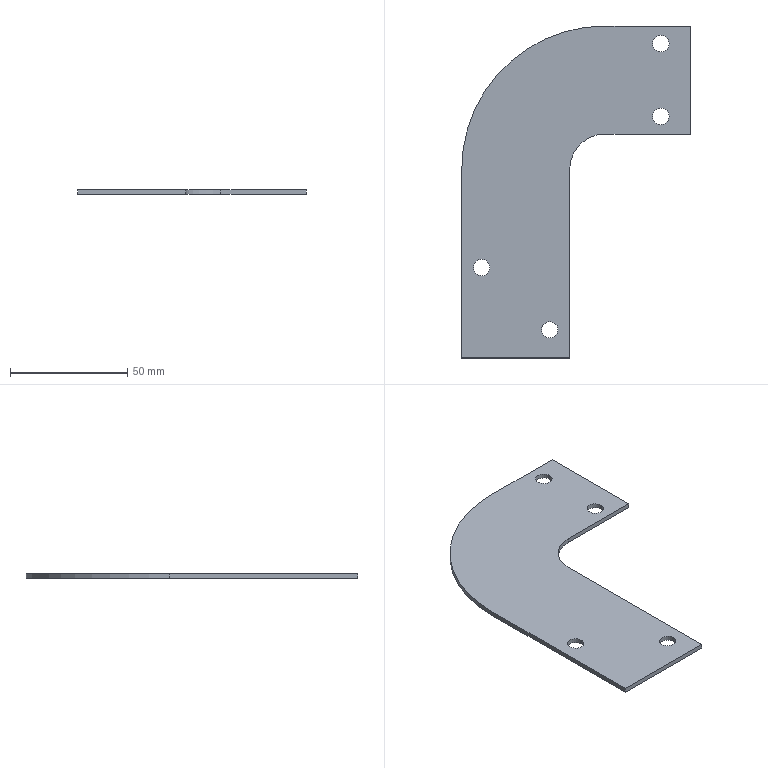Part | STEP file | 1_id806_x_t | 1 solid | 18 faces | box 97.332 x 141.374 x 2 mm | volume 15921 mm3 | cylinder 10 | plane 8 | commonest cylinder face diameters 7 x8 30 x1 122 x1
STEP:
#1=CARTESIAN_POINT('',(0.,0.,0.));
#2=DIRECTION('',(0.,0.,1.));
#3=DIRECTION('',(1.,0.,0.));
#4=AXIS2_PLACEMENT_3D('',#1,#2,#3);
#5=CARTESIAN_POINT('',(841.892,314.003,-88.));
#6=VERTEX_POINT('',#5);
#7=CARTESIAN_POINT('',(841.892,233.628,-88.));
#8=VERTEX_POINT('',#7);
#9=CARTESIAN_POINT('',(841.892,314.003,-88.));
#10=DIRECTION('',(0.,-1.,0.));
#11=VECTOR('',#10,1.);
#12=LINE('',#9,#11);
#13=CARTESIAN_POINT('',(902.892,314.003,-88.));
#14=DIRECTION('',(0.,0.,-1.));
#15=DIRECTION('',(-1.,0.,0.));
#16=AXIS2_PLACEMENT_3D('',#13,#14,#15);
#17=PLANE('',#16);
#18=CARTESIAN_POINT('',(61.,0.));
#19=DIRECTION('',(0.,-1.));
#20=VECTOR('',#19,1.);
#21=LINE('',#18,#20);
#22=(GEOMETRIC_REPRESENTATION_CONTEXT(2)PARAMETRIC_REPRESENTATION_CONTEXT()REPRESENTATION_CONTEXT('',''));
#23=DEFINITIONAL_REPRESENTATION('',(#21),#22);
#24=PCURVE('',#17,#23);
#25=CARTESIAN_POINT('',(841.892,225.628,-88.));
#26=DIRECTION('',(-1.,0.,0.));
#27=DIRECTION('',(0.,-1.,0.));
#28=AXIS2_PLACEMENT_3D('',#25,#26,#27);
#29=PLANE('',#28);
#30=CARTESIAN_POINT('',(-88.374,0.));
#31=DIRECTION('',(1.,0.));
#32=VECTOR('',#31,1.);
#33=LINE('',#30,#32);
#34=(GEOMETRIC_REPRESENTATION_CONTEXT(2)PARAMETRIC_REPRESENTATION_CONTEXT()REPRESENTATION_CONTEXT('',''));
#35=DEFINITIONAL_REPRESENTATION('',(#33),#34);
#36=PCURVE('',#29,#35);
#37=SURFACE_CURVE('',#12,(#24,#36),.PCURVE_S1.);
#38=EDGE_CURVE('',#6,#8,#37,.T.);
#39=ORIENTED_EDGE('',*,*,#38,.T.);
#40=CARTESIAN_POINT('',(887.892,233.628,-88.));
#41=VERTEX_POINT('',#40);
#42=CARTESIAN_POINT('',(841.892,233.628,-88.));
#43=DIRECTION('',(1.,0.,0.));
#44=VECTOR('',#43,1.);
#45=LINE('',#42,#44);
#46=CARTESIAN_POINT('',(61.,-80.374));
#47=DIRECTION('',(-1.,0.));
#48=VECTOR('',#47,1.);
#49=LINE('',#46,#48);
#50=(GEOMETRIC_REPRESENTATION_CONTEXT(2)PARAMETRIC_REPRESENTATION_CONTEXT()REPRESENTATION_CONTEXT('',''));
#51=DEFINITIONAL_REPRESENTATION('',(#49),#50);
#52=PCURVE('',#17,#51);
#53=CARTESIAN_POINT('',(887.892,233.628,-88.));
#54=DIRECTION('',(0.,-1.,0.));
#55=DIRECTION('',(0.,0.,1.));
#56=AXIS2_PLACEMENT_3D('',#53,#54,#55);
#57=PLANE('',#56);
#58=CARTESIAN_POINT('',(0.,46.));
#59=DIRECTION('',(0.,-1.));
#60=VECTOR('',#59,1.);
#61=LINE('',#58,#60);
#62=(GEOMETRIC_REPRESENTATION_CONTEXT(2)PARAMETRIC_REPRESENTATION_CONTEXT()REPRESENTATION_CONTEXT('',''));
#63=DEFINITIONAL_REPRESENTATION('',(#61),#62);
#64=PCURVE('',#57,#63);
#65=SURFACE_CURVE('',#45,(#52,#64),.PCURVE_S1.);
#66=EDGE_CURVE('',#8,#41,#65,.T.);
#67=ORIENTED_EDGE('',*,*,#66,.T.);
#68=CARTESIAN_POINT('',(887.892,314.003,-88.));
#69=VERTEX_POINT('',#68);
#70=CARTESIAN_POINT('',(887.892,233.628,-88.));
#71=DIRECTION('',(0.,1.,0.));
#72=VECTOR('',#71,1.);
#73=LINE('',#70,#72);
#74=CARTESIAN_POINT('',(15.,-80.374));
#75=DIRECTION('',(0.,1.));
#76=VECTOR('',#75,1.);
#77=LINE('',#74,#76);
#78=(GEOMETRIC_REPRESENTATION_CONTEXT(2)PARAMETRIC_REPRESENTATION_CONTEXT()REPRESENTATION_CONTEXT('',''));
#79=DEFINITIONAL_REPRESENTATION('',(#77),#78);
#80=PCURVE('',#17,#79);
#81=CARTESIAN_POINT('',(887.892,314.003,-88.));
#82=DIRECTION('',(1.,0.,0.));
#83=DIRECTION('',(0.,1.,0.));
#84=AXIS2_PLACEMENT_3D('',#81,#82,#83);
#85=PLANE('',#84);
#86=CARTESIAN_POINT('',(-80.374,0.));
#87=DIRECTION('',(1.,0.));
#88=VECTOR('',#87,1.);
#89=LINE('',#86,#88);
#90=(GEOMETRIC_REPRESENTATION_CONTEXT(2)PARAMETRIC_REPRESENTATION_CONTEXT()REPRESENTATION_CONTEXT('',''));
#91=DEFINITIONAL_REPRESENTATION('',(#89),#90);
#92=PCURVE('',#85,#91);
#93=SURFACE_CURVE('',#73,(#80,#92),.PCURVE_S1.);
#94=EDGE_CURVE('',#41,#69,#93,.T.);
#95=ORIENTED_EDGE('',*,*,#94,.T.);
#96=CARTESIAN_POINT('',(902.892,329.003,-88.));
#97=VERTEX_POINT('',#96);
#98=CARTESIAN_POINT('',(902.892,314.003,-88.));
#99=DIRECTION('',(0.,0.,-1.));
#100=DIRECTION('',(-1.,0.,0.));
#101=AXIS2_PLACEMENT_3D('',#98,#99,#100);
#102=CIRCLE('',#101,15.);
#103=CARTESIAN_POINT('',(0.,0.));
#104=DIRECTION('',(1.,0.));
#105=AXIS2_PLACEMENT_2D('',#103,#104);
#106=CIRCLE('',#105,15.);
#107=(GEOMETRIC_REPRESENTATION_CONTEXT(2)PARAMETRIC_REPRESENTATION_CONTEXT()REPRESENTATION_CONTEXT('',''));
#108=DEFINITIONAL_REPRESENTATION('',(#106),#107);
#109=PCURVE('',#17,#108);
#110=CARTESIAN_POINT('',(902.892,314.003,-88.));
#111=DIRECTION('',(0.,0.,-1.));
#112=DIRECTION('',(-1.,0.,0.));
#113=AXIS2_PLACEMENT_3D('',#110,#111,#112);
#114=CYLINDRICAL_SURFACE('',#113,15.);
#115=CARTESIAN_POINT('',(0.,0.));
#116=DIRECTION('',(1.,0.));
#117=VECTOR('',#116,1.);
#118=LINE('',#115,#117);
#119=(GEOMETRIC_REPRESENTATION_CONTEXT(2)PARAMETRIC_REPRESENTATION_CONTEXT()REPRESENTATION_CONTEXT('',''));
#120=DEFINITIONAL_REPRESENTATION('',(#118),#119);
#121=PCURVE('',#114,#120);
#122=SURFACE_CURVE('',#102,(#109,#121),.PCURVE_S1.);
#123=EDGE_CURVE('',#69,#97,#122,.T.);
#124=ORIENTED_EDGE('',*,*,#123,.T.);
#125=CARTESIAN_POINT('',(939.224,329.003,-88.));
#126=VERTEX_POINT('',#125);
#127=CARTESIAN_POINT('',(902.892,329.003,-88.));
#128=DIRECTION('',(1.,0.,0.));
#129=VECTOR('',#128,1.);
#130=LINE('',#127,#129);
#131=CARTESIAN_POINT('',(0.,15.));
#132=DIRECTION('',(-1.,0.));
#133=VECTOR('',#132,1.);
#134=LINE('',#131,#133);
#135=(GEOMETRIC_REPRESENTATION_CONTEXT(2)PARAMETRIC_REPRESENTATION_CONTEXT()REPRESENTATION_CONTEXT('',''));
#136=DEFINITIONAL_REPRESENTATION('',(#134),#135);
#137=PCURVE('',#17,#136);
#138=CARTESIAN_POINT('',(939.224,329.003,-88.));
#139=DIRECTION('',(0.,-1.,0.));
#140=DIRECTION('',(1.,0.,0.));
#141=AXIS2_PLACEMENT_3D('',#138,#139,#140);
#142=PLANE('',#141);
#143=CARTESIAN_POINT('',(-36.332,0.));
#144=DIRECTION('',(1.,0.));
#145=VECTOR('',#144,1.);
#146=LINE('',#143,#145);
#147=(GEOMETRIC_REPRESENTATION_CONTEXT(2)PARAMETRIC_REPRESENTATION_CONTEXT()REPRESENTATION_CONTEXT('',''));
#148=DEFINITIONAL_REPRESENTATION('',(#146),#147);
#149=PCURVE('',#142,#148);
#150=SURFACE_CURVE('',#130,(#137,#149),.PCURVE_S1.);
#151=EDGE_CURVE('',#97,#126,#150,.T.);
#152=ORIENTED_EDGE('',*,*,#151,.T.);
#153=CARTESIAN_POINT('',(939.224,375.003,-88.));
#154=VERTEX_POINT('',#153);
#155=CARTESIAN_POINT('',(939.224,329.003,-88.));
#156=DIRECTION('',(0.,1.,0.));
#157=VECTOR('',#156,1.);
#158=LINE('',#155,#157);
#159=CARTESIAN_POINT('',(-36.332,15.));
#160=DIRECTION('',(0.,1.));
#161=VECTOR('',#160,1.);
#162=LINE('',#159,#161);
#163=(GEOMETRIC_REPRESENTATION_CONTEXT(2)PARAMETRIC_REPRESENTATION_CONTEXT()REPRESENTATION_CONTEXT('',''));
#164=DEFINITIONAL_REPRESENTATION('',(#162),#163);
#165=PCURVE('',#17,#164);
#166=CARTESIAN_POINT('',(939.224,375.003,-88.));
#167=DIRECTION('',(1.,0.,0.));
#168=DIRECTION('',(0.,1.,0.));
#169=AXIS2_PLACEMENT_3D('',#166,#167,#168);
#170=PLANE('',#169);
#171=CARTESIAN_POINT('',(-46.,0.));
#172=DIRECTION('',(1.,0.));
#173=VECTOR('',#172,1.);
#174=LINE('',#171,#173);
#175=(GEOMETRIC_REPRESENTATION_CONTEXT(2)PARAMETRIC_REPRESENTATION_CONTEXT()REPRESENTATION_CONTEXT('',''));
#176=DEFINITIONAL_REPRESENTATION('',(#174),#175);
#177=PCURVE('',#170,#176);
#178=SURFACE_CURVE('',#158,(#165,#177),.PCURVE_S1.);
#179=EDGE_CURVE('',#126,#154,#178,.T.);
#180=ORIENTED_EDGE('',*,*,#179,.T.);
#181=CARTESIAN_POINT('',(902.892,375.003,-88.));
#182=VERTEX_POINT('',#181);
#183=CARTESIAN_POINT('',(939.224,375.003,-88.));
#184=DIRECTION('',(-1.,0.,0.));
#185=VECTOR('',#184,1.);
#186=LINE('',#183,#185);
#187=CARTESIAN_POINT('',(-36.332,61.));
#188=DIRECTION('',(1.,0.));
#189=VECTOR('',#188,1.);
#190=LINE('',#187,#189);
#191=(GEOMETRIC_REPRESENTATION_CONTEXT(2)PARAMETRIC_REPRESENTATION_CONTEXT()REPRESENTATION_CONTEXT('',''));
#192=DEFINITIONAL_REPRESENTATION('',(#190),#191);
#193=PCURVE('',#17,#192);
#194=CARTESIAN_POINT('',(902.892,375.003,-88.));
#195=DIRECTION('',(0.,1.,0.));
#196=DIRECTION('',(0.,0.,-1.));
#197=AXIS2_PLACEMENT_3D('',#194,#195,#196);
#198=PLANE('',#197);
#199=CARTESIAN_POINT('',(0.,-36.332));
#200=DIRECTION('',(0.,1.));
#201=VECTOR('',#200,1.);
#202=LINE('',#199,#201);
#203=(GEOMETRIC_REPRESENTATION_CONTEXT(2)PARAMETRIC_REPRESENTATION_CONTEXT()REPRESENTATION_CONTEXT('',''));
#204=DEFINITIONAL_REPRESENTATION('',(#202),#203);
#205=PCURVE('',#198,#204);
#206=SURFACE_CURVE('',#186,(#193,#205),.PCURVE_S1.);
#207=EDGE_CURVE('',#154,#182,#206,.T.);
#208=ORIENTED_EDGE('',*,*,#207,.T.);
#209=CARTESIAN_POINT('',(902.892,314.003,-88.));
#210=DIRECTION('',(0.,0.,1.));
#211=DIRECTION('',(0.,1.,0.));
#212=AXIS2_PLACEMENT_3D('',#209,#210,#211);
#213=CIRCLE('',#212,61.);
#214=CARTESIAN_POINT('',(0.,61.));
#215=CARTESIAN_POINT('',(105.655,61.));
#216=CARTESIAN_POINT('',(52.828,-30.5));
#217=CARTESIAN_POINT('',(0.,-122.));
#218=CARTESIAN_POINT('',(-52.828,-30.5));
#219=CARTESIAN_POINT('',(-105.655,61.));
#220=CARTESIAN_POINT('',(0.,61.));
#221=(BOUNDED_CURVE()B_SPLINE_CURVE(2,(#214,#215,#216,#217,#218,#219,#220),.UNSPECIFIED.,.T.,.F.)B_SPLINE_CURVE_WITH_KNOTS((1,2,2,2,2,1),(-2.094,0.,2.094,4.189,6.283,8.378),.UNSPECIFIED.)CURVE()GEOMETRIC_REPRESENTATION_ITEM()RATIONAL_B_SPLINE_CURVE((1.,0.5,1.,0.5,1.,0.5,1.))REPRESENTATION_ITEM(''));
#222=(GEOMETRIC_REPRESENTATION_CONTEXT(2)PARAMETRIC_REPRESENTATION_CONTEXT()REPRESENTATION_CONTEXT('',''));
#223=DEFINITIONAL_REPRESENTATION('',(#221),#222);
#224=PCURVE('',#17,#223);
#225=CARTESIAN_POINT('',(902.892,314.003,-88.));
#226=DIRECTION('',(0.,0.,-1.));
#227=DIRECTION('',(-1.,0.,0.));
#228=AXIS2_PLACEMENT_3D('',#225,#226,#227);
#229=CYLINDRICAL_SURFACE('',#228,61.);
#230=CARTESIAN_POINT('',(1.571,0.));
#231=DIRECTION('',(-1.,0.));
#232=VECTOR('',#231,1.);
#233=LINE('',#230,#232);
#234=(GEOMETRIC_REPRESENTATION_CONTEXT(2)PARAMETRIC_REPRESENTATION_CONTEXT()REPRESENTATION_CONTEXT('',''));
#235=DEFINITIONAL_REPRESENTATION('',(#233),#234);
#236=PCURVE('',#229,#235);
#237=SURFACE_CURVE('',#213,(#224,#236),.PCURVE_S1.);
#238=EDGE_CURVE('',#182,#6,#237,.T.);
#239=ORIENTED_EDGE('',*,*,#238,.T.);
#240=EDGE_LOOP('',(#39,#67,#95,#124,#152,#180,#208,#239));
#241=FACE_BOUND('',#240,.T.);
#242=CARTESIAN_POINT('',(853.892,272.128,-88.));
#243=VERTEX_POINT('',#242);
#244=CARTESIAN_POINT('',(846.892,272.128,-88.));
#245=VERTEX_POINT('',#244);
#246=CARTESIAN_POINT('',(850.392,272.128,-88.));
#247=DIRECTION('',(0.,0.,-1.));
#248=DIRECTION('',(1.,0.,0.));
#249=AXIS2_PLACEMENT_3D('',#246,#247,#248);
#250=CIRCLE('',#249,3.5);
#251=CARTESIAN_POINT('',(52.5,-41.874));
#252=DIRECTION('',(-1.,0.));
#253=AXIS2_PLACEMENT_2D('',#251,#252);
#254=CIRCLE('',#253,3.5);
#255=(GEOMETRIC_REPRESENTATION_CONTEXT(2)PARAMETRIC_REPRESENTATION_CONTEXT()REPRESENTATION_CONTEXT('',''));
#256=DEFINITIONAL_REPRESENTATION('',(#254),#255);
#257=PCURVE('',#17,#256);
#258=CARTESIAN_POINT('',(850.392,272.128,-88.));
#259=DIRECTION('',(0.,0.,-1.));
#260=DIRECTION('',(1.,0.,0.));
#261=AXIS2_PLACEMENT_3D('',#258,#259,#260);
#262=CYLINDRICAL_SURFACE('',#261,3.5);
#263=CARTESIAN_POINT('',(0.,0.));
#264=DIRECTION('',(1.,0.));
#265=VECTOR('',#264,1.);
#266=LINE('',#263,#265);
#267=(GEOMETRIC_REPRESENTATION_CONTEXT(2)PARAMETRIC_REPRESENTATION_CONTEXT()REPRESENTATION_CONTEXT('',''));
#268=DEFINITIONAL_REPRESENTATION('',(#266),#267);
#269=PCURVE('',#262,#268);
#270=SURFACE_CURVE('',#250,(#257,#269),.PCURVE_S1.);
#271=EDGE_CURVE('',#243,#245,#270,.T.);
#272=ORIENTED_EDGE('',*,*,#271,.T.);
#273=CARTESIAN_POINT('',(850.392,272.128,-88.));
#274=DIRECTION('',(0.,0.,-1.));
#275=DIRECTION('',(-1.,0.,0.));
#276=AXIS2_PLACEMENT_3D('',#273,#274,#275);
#277=CIRCLE('',#276,3.5);
#278=CARTESIAN_POINT('',(52.5,-41.874));
#279=DIRECTION('',(1.,0.));
#280=AXIS2_PLACEMENT_2D('',#278,#279);
#281=CIRCLE('',#280,3.5);
#282=(GEOMETRIC_REPRESENTATION_CONTEXT(2)PARAMETRIC_REPRESENTATION_CONTEXT()REPRESENTATION_CONTEXT('',''));
#283=DEFINITIONAL_REPRESENTATION('',(#281),#282);
#284=PCURVE('',#17,#283);
#285=CARTESIAN_POINT('',(850.392,272.128,-88.));
#286=DIRECTION('',(0.,0.,-1.));
#287=DIRECTION('',(1.,0.,0.));
#288=AXIS2_PLACEMENT_3D('',#285,#286,#287);
#289=CYLINDRICAL_SURFACE('',#288,3.5);
#290=CARTESIAN_POINT('',(3.142,0.));
#291=DIRECTION('',(1.,0.));
#292=VECTOR('',#291,1.);
#293=LINE('',#290,#292);
#294=(GEOMETRIC_REPRESENTATION_CONTEXT(2)PARAMETRIC_REPRESENTATION_CONTEXT()REPRESENTATION_CONTEXT('',''));
#295=DEFINITIONAL_REPRESENTATION('',(#293),#294);
#296=PCURVE('',#289,#295);
#297=SURFACE_CURVE('',#277,(#284,#296),.PCURVE_S1.);
#298=EDGE_CURVE('',#245,#243,#297,.T.);
#299=ORIENTED_EDGE('',*,*,#298,.T.);
#300=EDGE_LOOP('',(#272,#299));
#301=FACE_BOUND('',#300,.T.);
#302=CARTESIAN_POINT('',(875.892,245.628,-88.));
#303=VERTEX_POINT('',#302);
#304=CARTESIAN_POINT('',(882.892,245.628,-88.));
#305=VERTEX_POINT('',#304);
#306=CARTESIAN_POINT('',(879.392,245.628,-88.));
#307=DIRECTION('',(0.,0.,-1.));
#308=DIRECTION('',(-1.,0.,0.));
#309=AXIS2_PLACEMENT_3D('',#306,#307,#308);
#310=CIRCLE('',#309,3.5);
#311=CARTESIAN_POINT('',(23.5,-68.374));
#312=DIRECTION('',(1.,0.));
#313=AXIS2_PLACEMENT_2D('',#311,#312);
#314=CIRCLE('',#313,3.5);
#315=(GEOMETRIC_REPRESENTATION_CONTEXT(2)PARAMETRIC_REPRESENTATION_CONTEXT()REPRESENTATION_CONTEXT('',''));
#316=DEFINITIONAL_REPRESENTATION('',(#314),#315);
#317=PCURVE('',#17,#316);
#318=CARTESIAN_POINT('',(879.392,245.628,-88.));
#319=DIRECTION('',(0.,0.,-1.));
#320=DIRECTION('',(-1.,0.,0.));
#321=AXIS2_PLACEMENT_3D('',#318,#319,#320);
#322=CYLINDRICAL_SURFACE('',#321,3.5);
#323=CARTESIAN_POINT('',(0.,0.));
#324=DIRECTION('',(1.,0.));
#325=VECTOR('',#324,1.);
#326=LINE('',#323,#325);
#327=(GEOMETRIC_REPRESENTATION_CONTEXT(2)PARAMETRIC_REPRESENTATION_CONTEXT()REPRESENTATION_CONTEXT('',''));
#328=DEFINITIONAL_REPRESENTATION('',(#326),#327);
#329=PCURVE('',#322,#328);
#330=SURFACE_CURVE('',#310,(#317,#329),.PCURVE_S1.);
#331=EDGE_CURVE('',#303,#305,#330,.T.);
#332=ORIENTED_EDGE('',*,*,#331,.T.);
#333=CARTESIAN_POINT('',(879.392,245.628,-88.));
#334=DIRECTION('',(0.,0.,-1.));
#335=DIRECTION('',(1.,0.,0.));
#336=AXIS2_PLACEMENT_3D('',#333,#334,#335);
#337=CIRCLE('',#336,3.5);
#338=CARTESIAN_POINT('',(23.5,-68.374));
#339=DIRECTION('',(-1.,0.));
#340=AXIS2_PLACEMENT_2D('',#338,#339);
#341=CIRCLE('',#340,3.5);
#342=(GEOMETRIC_REPRESENTATION_CONTEXT(2)PARAMETRIC_REPRESENTATION_CONTEXT()REPRESENTATION_CONTEXT('',''));
#343=DEFINITIONAL_REPRESENTATION('',(#341),#342);
#344=PCURVE('',#17,#343);
#345=CARTESIAN_POINT('',(879.392,245.628,-88.));
#346=DIRECTION('',(0.,0.,-1.));
#347=DIRECTION('',(-1.,0.,0.));
#348=AXIS2_PLACEMENT_3D('',#345,#346,#347);
#349=CYLINDRICAL_SURFACE('',#348,3.5);
#350=CARTESIAN_POINT('',(3.142,0.));
#351=DIRECTION('',(1.,0.));
#352=VECTOR('',#351,1.);
#353=LINE('',#350,#352);
#354=(GEOMETRIC_REPRESENTATION_CONTEXT(2)PARAMETRIC_REPRESENTATION_CONTEXT()REPRESENTATION_CONTEXT('',''));
#355=DEFINITIONAL_REPRESENTATION('',(#353),#354);
#356=PCURVE('',#349,#355);
#357=SURFACE_CURVE('',#337,(#344,#356),.PCURVE_S1.);
#358=EDGE_CURVE('',#305,#303,#357,.T.);
#359=ORIENTED_EDGE('',*,*,#358,.T.);
#360=EDGE_LOOP('',(#332,#359));
#361=FACE_BOUND('',#360,.T.);
#362=CARTESIAN_POINT('',(923.224,336.503,-88.));
#363=VERTEX_POINT('',#362);
#364=CARTESIAN_POINT('',(930.224,336.503,-88.));
#365=VERTEX_POINT('',#364);
#366=CARTESIAN_POINT('',(926.724,336.503,-88.));
#367=DIRECTION('',(0.,0.,-1.));
#368=DIRECTION('',(-1.,0.,0.));
#369=AXIS2_PLACEMENT_3D('',#366,#367,#368);
#370=CIRCLE('',#369,3.5);
#371=CARTESIAN_POINT('',(-23.832,22.5));
#372=DIRECTION('',(1.,0.));
#373=AXIS2_PLACEMENT_2D('',#371,#372);
#374=CIRCLE('',#373,3.5);
#375=(GEOMETRIC_REPRESENTATION_CONTEXT(2)PARAMETRIC_REPRESENTATION_CONTEXT()REPRESENTATION_CONTEXT('',''));
#376=DEFINITIONAL_REPRESENTATION('',(#374),#375);
#377=PCURVE('',#17,#376);
#378=CARTESIAN_POINT('',(926.724,336.503,-88.));
#379=DIRECTION('',(0.,0.,-1.));
#380=DIRECTION('',(-1.,0.,0.));
#381=AXIS2_PLACEMENT_3D('',#378,#379,#380);
#382=CYLINDRICAL_SURFACE('',#381,3.5);
#383=CARTESIAN_POINT('',(0.,0.));
#384=DIRECTION('',(1.,0.));
#385=VECTOR('',#384,1.);
#386=LINE('',#383,#385);
#387=(GEOMETRIC_REPRESENTATION_CONTEXT(2)PARAMETRIC_REPRESENTATION_CONTEXT()REPRESENTATION_CONTEXT('',''));
#388=DEFINITIONAL_REPRESENTATION('',(#386),#387);
#389=PCURVE('',#382,#388);
#390=SURFACE_CURVE('',#370,(#377,#389),.PCURVE_S1.);
#391=EDGE_CURVE('',#363,#365,#390,.T.);
#392=ORIENTED_EDGE('',*,*,#391,.T.);
#393=CARTESIAN_POINT('',(926.724,336.503,-88.));
#394=DIRECTION('',(0.,0.,-1.));
#395=DIRECTION('',(1.,0.,0.));
#396=AXIS2_PLACEMENT_3D('',#393,#394,#395);
#397=CIRCLE('',#396,3.5);
#398=CARTESIAN_POINT('',(-23.832,22.5));
#399=DIRECTION('',(-1.,0.));
#400=AXIS2_PLACEMENT_2D('',#398,#399);
#401=CIRCLE('',#400,3.5);
#402=(GEOMETRIC_REPRESENTATION_CONTEXT(2)PARAMETRIC_REPRESENTATION_CONTEXT()REPRESENTATION_CONTEXT('',''));
#403=DEFINITIONAL_REPRESENTATION('',(#401),#402);
#404=PCURVE('',#17,#403);
#405=CARTESIAN_POINT('',(926.724,336.503,-88.));
#406=DIRECTION('',(0.,0.,-1.));
#407=DIRECTION('',(-1.,0.,0.));
#408=AXIS2_PLACEMENT_3D('',#405,#406,#407);
#409=CYLINDRICAL_SURFACE('',#408,3.5);
#410=CARTESIAN_POINT('',(3.142,0.));
#411=DIRECTION('',(1.,0.));
#412=VECTOR('',#411,1.);
#413=LINE('',#410,#412);
#414=(GEOMETRIC_REPRESENTATION_CONTEXT(2)PARAMETRIC_REPRESENTATION_CONTEXT()REPRESENTATION_CONTEXT('',''));
#415=DEFINITIONAL_REPRESENTATION('',(#413),#414);
#416=PCURVE('',#409,#415);
#417=SURFACE_CURVE('',#397,(#404,#416),.PCURVE_S1.);
#418=EDGE_CURVE('',#365,#363,#417,.T.);
#419=ORIENTED_EDGE('',*,*,#418,.T.);
#420=EDGE_LOOP('',(#392,#419));
#421=FACE_BOUND('',#420,.T.);
#422=CARTESIAN_POINT('',(923.224,367.503,-88.));
#423=VERTEX_POINT('',#422);
#424=CARTESIAN_POINT('',(930.224,367.503,-88.));
#425=VERTEX_POINT('',#424);
#426=CARTESIAN_POINT('',(926.724,367.503,-88.));
#427=DIRECTION('',(0.,0.,-1.));
#428=DIRECTION('',(-1.,0.,0.));
#429=AXIS2_PLACEMENT_3D('',#426,#427,#428);
#430=CIRCLE('',#429,3.5);
#431=CARTESIAN_POINT('',(-23.832,53.5));
#432=DIRECTION('',(1.,0.));
#433=AXIS2_PLACEMENT_2D('',#431,#432);
#434=CIRCLE('',#433,3.5);
#435=(GEOMETRIC_REPRESENTATION_CONTEXT(2)PARAMETRIC_REPRESENTATION_CONTEXT()REPRESENTATION_CONTEXT('',''));
#436=DEFINITIONAL_REPRESENTATION('',(#434),#435);
#437=PCURVE('',#17,#436);
#438=CARTESIAN_POINT('',(926.724,367.503,-88.));
#439=DIRECTION('',(0.,0.,-1.));
#440=DIRECTION('',(-1.,0.,0.));
#441=AXIS2_PLACEMENT_3D('',#438,#439,#440);
#442=CYLINDRICAL_SURFACE('',#441,3.5);
#443=CARTESIAN_POINT('',(0.,0.));
#444=DIRECTION('',(1.,0.));
#445=VECTOR('',#444,1.);
#446=LINE('',#443,#445);
#447=(GEOMETRIC_REPRESENTATION_CONTEXT(2)PARAMETRIC_REPRESENTATION_CONTEXT()REPRESENTATION_CONTEXT('',''));
#448=DEFINITIONAL_REPRESENTATION('',(#446),#447);
#449=PCURVE('',#442,#448);
#450=SURFACE_CURVE('',#430,(#437,#449),.PCURVE_S1.);
#451=EDGE_CURVE('',#423,#425,#450,.T.);
#452=ORIENTED_EDGE('',*,*,#451,.T.);
#453=CARTESIAN_POINT('',(926.724,367.503,-88.));
#454=DIRECTION('',(0.,0.,-1.));
#455=DIRECTION('',(1.,0.,0.));
#456=AXIS2_PLACEMENT_3D('',#453,#454,#455);
#457=CIRCLE('',#456,3.5);
#458=CARTESIAN_POINT('',(-23.832,53.5));
#459=DIRECTION('',(-1.,0.));
#460=AXIS2_PLACEMENT_2D('',#458,#459);
#461=CIRCLE('',#460,3.5);
#462=(GEOMETRIC_REPRESENTATION_CONTEXT(2)PARAMETRIC_REPRESENTATION_CONTEXT()REPRESENTATION_CONTEXT('',''));
#463=DEFINITIONAL_REPRESENTATION('',(#461),#462);
#464=PCURVE('',#17,#463);
#465=CARTESIAN_POINT('',(926.724,367.503,-88.));
#466=DIRECTION('',(0.,0.,-1.));
#467=DIRECTION('',(-1.,0.,0.));
#468=AXIS2_PLACEMENT_3D('',#465,#466,#467);
#469=CYLINDRICAL_SURFACE('',#468,3.5);
#470=CARTESIAN_POINT('',(3.142,0.));
#471=DIRECTION('',(1.,0.));
#472=VECTOR('',#471,1.);
#473=LINE('',#470,#472);
#474=(GEOMETRIC_REPRESENTATION_CONTEXT(2)PARAMETRIC_REPRESENTATION_CONTEXT()REPRESENTATION_CONTEXT('',''));
#475=DEFINITIONAL_REPRESENTATION('',(#473),#474);
#476=PCURVE('',#469,#475);
#477=SURFACE_CURVE('',#457,(#464,#476),.PCURVE_S1.);
#478=EDGE_CURVE('',#425,#423,#477,.T.);
#479=ORIENTED_EDGE('',*,*,#478,.T.);
#480=EDGE_LOOP('',(#452,#479));
#481=FACE_BOUND('',#480,.T.);
#482=ADVANCED_FACE('',(#241,#301,#361,#421,#481),#17,.F.);
#483=CARTESIAN_POINT('',(853.892,272.128,-90.));
#484=VERTEX_POINT('',#483);
#485=CARTESIAN_POINT('',(846.892,272.128,-90.));
#486=VERTEX_POINT('',#485);
#487=CARTESIAN_POINT('',(850.392,272.128,-90.));
#488=DIRECTION('',(0.,0.,1.));
#489=DIRECTION('',(1.,0.,0.));
#490=AXIS2_PLACEMENT_3D('',#487,#488,#489);
#491=CIRCLE('',#490,3.5);
#492=CARTESIAN_POINT('',(6.283,2.));
#493=DIRECTION('',(-1.,0.));
#494=VECTOR('',#493,1.);
#495=LINE('',#492,#494);
#496=(GEOMETRIC_REPRESENTATION_CONTEXT(2)PARAMETRIC_REPRESENTATION_CONTEXT()REPRESENTATION_CONTEXT('',''));
#497=DEFINITIONAL_REPRESENTATION('',(#495),#496);
#498=PCURVE('',#289,#497);
#499=CARTESIAN_POINT('',(902.892,314.003,-90.));
#500=DIRECTION('',(0.,0.,-1.));
#501=DIRECTION('',(-1.,0.,0.));
#502=AXIS2_PLACEMENT_3D('',#499,#500,#501);
#503=PLANE('',#502);
#504=CARTESIAN_POINT('',(49.,-41.874));
#505=CARTESIAN_POINT('',(49.,-35.812));
#506=CARTESIAN_POINT('',(54.25,-38.843));
#507=CARTESIAN_POINT('',(59.5,-41.874));
#508=CARTESIAN_POINT('',(54.25,-44.905));
#509=CARTESIAN_POINT('',(49.,-47.936));
#510=CARTESIAN_POINT('',(49.,-41.874));
#511=(BOUNDED_CURVE()B_SPLINE_CURVE(2,(#504,#505,#506,#507,#508,#509,#510),.UNSPECIFIED.,.T.,.F.)B_SPLINE_CURVE_WITH_KNOTS((1,2,2,2,2,1),(-2.094,0.,2.094,4.189,6.283,8.378),.UNSPECIFIED.)CURVE()GEOMETRIC_REPRESENTATION_ITEM()RATIONAL_B_SPLINE_CURVE((1.,0.5,1.,0.5,1.,0.5,1.))REPRESENTATION_ITEM(''));
#512=(GEOMETRIC_REPRESENTATION_CONTEXT(2)PARAMETRIC_REPRESENTATION_CONTEXT()REPRESENTATION_CONTEXT('',''));
#513=DEFINITIONAL_REPRESENTATION('',(#511),#512);
#514=PCURVE('',#503,#513);
#515=SURFACE_CURVE('',#491,(#498,#514),.PCURVE_S1.);
#516=EDGE_CURVE('',#484,#486,#515,.T.);
#517=ORIENTED_EDGE('',*,*,#516,.T.);
#518=CARTESIAN_POINT('',(846.892,272.128,-88.));
#519=DIRECTION('',(0.,0.,-1.));
#520=VECTOR('',#519,1.);
#521=LINE('',#518,#520);
#522=CARTESIAN_POINT('',(3.142,0.));
#523=DIRECTION('',(0.,1.));
#524=VECTOR('',#523,1.);
#525=LINE('',#522,#524);
#526=(GEOMETRIC_REPRESENTATION_CONTEXT(2)PARAMETRIC_REPRESENTATION_CONTEXT()REPRESENTATION_CONTEXT('',''));
#527=DEFINITIONAL_REPRESENTATION('',(#525),#526);
#528=PCURVE('',#289,#527);
#529=CARTESIAN_POINT('',(3.142,0.));
#530=DIRECTION('',(0.,1.));
#531=VECTOR('',#530,1.);
#532=LINE('',#529,#531);
#533=(GEOMETRIC_REPRESENTATION_CONTEXT(2)PARAMETRIC_REPRESENTATION_CONTEXT()REPRESENTATION_CONTEXT('',''));
#534=DEFINITIONAL_REPRESENTATION('',(#532),#533);
#535=PCURVE('',#262,#534);
#536=SURFACE_CURVE('',#521,(#528,#535),.PCURVE_S1.);
#537=EDGE_CURVE('',#245,#486,#536,.T.);
#538=ORIENTED_EDGE('',*,*,#537,.F.);
#539=ORIENTED_EDGE('',*,*,#298,.T.);
#540=CARTESIAN_POINT('',(853.892,272.128,-88.));
#541=DIRECTION('',(0.,0.,1.));
#542=VECTOR('',#541,1.);
#543=LINE('',#540,#542);
#544=CARTESIAN_POINT('',(6.283,0.));
#545=DIRECTION('',(0.,-1.));
#546=VECTOR('',#545,1.);
#547=LINE('',#544,#546);
#548=(GEOMETRIC_REPRESENTATION_CONTEXT(2)PARAMETRIC_REPRESENTATION_CONTEXT()REPRESENTATION_CONTEXT('',''));
#549=DEFINITIONAL_REPRESENTATION('',(#547),#548);
#550=PCURVE('',#289,#549);
#551=CARTESIAN_POINT('',(0.,0.));
#552=DIRECTION('',(0.,-1.));
#553=VECTOR('',#552,1.);
#554=LINE('',#551,#553);
#555=(GEOMETRIC_REPRESENTATION_CONTEXT(2)PARAMETRIC_REPRESENTATION_CONTEXT()REPRESENTATION_CONTEXT('',''));
#556=DEFINITIONAL_REPRESENTATION('',(#554),#555);
#557=PCURVE('',#262,#556);
#558=SURFACE_CURVE('',#543,(#550,#557),.PCURVE_S1.);
#559=EDGE_CURVE('',#484,#243,#558,.T.);
#560=ORIENTED_EDGE('',*,*,#559,.F.);
#561=EDGE_LOOP('',(#517,#538,#539,#560));
#562=FACE_BOUND('',#561,.F.);
#563=ADVANCED_FACE('',(#562),#289,.F.);
#564=CARTESIAN_POINT('',(939.224,375.003,-90.));
#565=VERTEX_POINT('',#564);
#566=CARTESIAN_POINT('',(902.892,375.003,-90.));
#567=VERTEX_POINT('',#566);
#568=CARTESIAN_POINT('',(939.224,375.003,-90.));
#569=DIRECTION('',(-1.,0.,0.));
#570=VECTOR('',#569,1.);
#571=LINE('',#568,#570);
#572=CARTESIAN_POINT('',(-36.332,61.));
#573=DIRECTION('',(1.,0.));
#574=VECTOR('',#573,1.);
#575=LINE('',#572,#574);
#576=(GEOMETRIC_REPRESENTATION_CONTEXT(2)PARAMETRIC_REPRESENTATION_CONTEXT()REPRESENTATION_CONTEXT('',''));
#577=DEFINITIONAL_REPRESENTATION('',(#575),#576);
#578=PCURVE('',#503,#577);
#579=CARTESIAN_POINT('',(2.,-36.332));
#580=DIRECTION('',(0.,1.));
#581=VECTOR('',#580,1.);
#582=LINE('',#579,#581);
#583=(GEOMETRIC_REPRESENTATION_CONTEXT(2)PARAMETRIC_REPRESENTATION_CONTEXT()REPRESENTATION_CONTEXT('',''));
#584=DEFINITIONAL_REPRESENTATION('',(#582),#583);
#585=PCURVE('',#198,#584);
#586=SURFACE_CURVE('',#571,(#578,#585),.PCURVE_S1.);
#587=EDGE_CURVE('',#565,#567,#586,.T.);
#588=ORIENTED_EDGE('',*,*,#587,.F.);
#589=CARTESIAN_POINT('',(939.224,329.003,-90.));
#590=VERTEX_POINT('',#589);
#591=CARTESIAN_POINT('',(939.224,329.003,-90.));
#592=DIRECTION('',(0.,1.,0.));
#593=VECTOR('',#592,1.);
#594=LINE('',#591,#593);
#595=CARTESIAN_POINT('',(-36.332,15.));
#596=DIRECTION('',(0.,1.));
#597=VECTOR('',#596,1.);
#598=LINE('',#595,#597);
#599=(GEOMETRIC_REPRESENTATION_CONTEXT(2)PARAMETRIC_REPRESENTATION_CONTEXT()REPRESENTATION_CONTEXT('',''));
#600=DEFINITIONAL_REPRESENTATION('',(#598),#599);
#601=PCURVE('',#503,#600);
#602=CARTESIAN_POINT('',(-46.,-2.));
#603=DIRECTION('',(1.,0.));
#604=VECTOR('',#603,1.);
#605=LINE('',#602,#604);
#606=(GEOMETRIC_REPRESENTATION_CONTEXT(2)PARAMETRIC_REPRESENTATION_CONTEXT()REPRESENTATION_CONTEXT('',''));
#607=DEFINITIONAL_REPRESENTATION('',(#605),#606);
#608=PCURVE('',#170,#607);
#609=SURFACE_CURVE('',#594,(#601,#608),.PCURVE_S1.);
#610=EDGE_CURVE('',#590,#565,#609,.T.);
#611=ORIENTED_EDGE('',*,*,#610,.F.);
#612=CARTESIAN_POINT('',(902.892,329.003,-90.));
#613=VERTEX_POINT('',#612);
#614=CARTESIAN_POINT('',(902.892,329.003,-90.));
#615=DIRECTION('',(1.,0.,0.));
#616=VECTOR('',#615,1.);
#617=LINE('',#614,#616);
#618=CARTESIAN_POINT('',(0.,15.));
#619=DIRECTION('',(-1.,0.));
#620=VECTOR('',#619,1.);
#621=LINE('',#618,#620);
#622=(GEOMETRIC_REPRESENTATION_CONTEXT(2)PARAMETRIC_REPRESENTATION_CONTEXT()REPRESENTATION_CONTEXT('',''));
#623=DEFINITIONAL_REPRESENTATION('',(#621),#622);
#624=PCURVE('',#503,#623);
#625=CARTESIAN_POINT('',(-36.332,-2.));
#626=DIRECTION('',(1.,0.));
#627=VECTOR('',#626,1.);
#628=LINE('',#625,#627);
#629=(GEOMETRIC_REPRESENTATION_CONTEXT(2)PARAMETRIC_REPRESENTATION_CONTEXT()REPRESENTATION_CONTEXT('',''));
#630=DEFINITIONAL_REPRESENTATION('',(#628),#629);
#631=PCURVE('',#142,#630);
#632=SURFACE_CURVE('',#617,(#624,#631),.PCURVE_S1.);
#633=EDGE_CURVE('',#613,#590,#632,.T.);
#634=ORIENTED_EDGE('',*,*,#633,.F.);
#635=CARTESIAN_POINT('',(887.892,314.003,-90.));
#636=VERTEX_POINT('',#635);
#637=CARTESIAN_POINT('',(902.892,314.003,-90.));
#638=DIRECTION('',(0.,0.,1.));
#639=DIRECTION('',(0.,1.,0.));
#640=AXIS2_PLACEMENT_3D('',#637,#638,#639);
#641=CIRCLE('',#640,15.);
#642=CARTESIAN_POINT('',(0.,15.));
#643=CARTESIAN_POINT('',(25.981,15.));
#644=CARTESIAN_POINT('',(12.99,-7.5));
#645=CARTESIAN_POINT('',(0.,-30.));
#646=CARTESIAN_POINT('',(-12.99,-7.5));
#647=CARTESIAN_POINT('',(-25.981,15.));
#648=CARTESIAN_POINT('',(0.,15.));
#649=(BOUNDED_CURVE()B_SPLINE_CURVE(2,(#642,#643,#644,#645,#646,#647,#648),.UNSPECIFIED.,.T.,.F.)B_SPLINE_CURVE_WITH_KNOTS((1,2,2,2,2,1),(-2.094,0.,2.094,4.189,6.283,8.378),.UNSPECIFIED.)CURVE()GEOMETRIC_REPRESENTATION_ITEM()RATIONAL_B_SPLINE_CURVE((1.,0.5,1.,0.5,1.,0.5,1.))REPRESENTATION_ITEM(''));
#650=(GEOMETRIC_REPRESENTATION_CONTEXT(2)PARAMETRIC_REPRESENTATION_CONTEXT()REPRESENTATION_CONTEXT('',''));
#651=DEFINITIONAL_REPRESENTATION('',(#649),#650);
#652=PCURVE('',#503,#651);
#653=CARTESIAN_POINT('',(1.571,2.));
#654=DIRECTION('',(-1.,0.));
#655=VECTOR('',#654,1.);
#656=LINE('',#653,#655);
#657=(GEOMETRIC_REPRESENTATION_CONTEXT(2)PARAMETRIC_REPRESENTATION_CONTEXT()REPRESENTATION_CONTEXT('',''));
#658=DEFINITIONAL_REPRESENTATION('',(#656),#657);
#659=PCURVE('',#114,#658);
#660=SURFACE_CURVE('',#641,(#652,#659),.PCURVE_S1.);
#661=EDGE_CURVE('',#613,#636,#660,.T.);
#662=ORIENTED_EDGE('',*,*,#661,.T.);
#663=CARTESIAN_POINT('',(887.892,233.628,-90.));
#664=VERTEX_POINT('',#663);
#665=CARTESIAN_POINT('',(887.892,233.628,-90.));
#666=DIRECTION('',(0.,1.,0.));
#667=VECTOR('',#666,1.);
#668=LINE('',#665,#667);
#669=CARTESIAN_POINT('',(15.,-80.374));
#670=DIRECTION('',(0.,1.));
#671=VECTOR('',#670,1.);
#672=LINE('',#669,#671);
#673=(GEOMETRIC_REPRESENTATION_CONTEXT(2)PARAMETRIC_REPRESENTATION_CONTEXT()REPRESENTATION_CONTEXT('',''));
#674=DEFINITIONAL_REPRESENTATION('',(#672),#673);
#675=PCURVE('',#503,#674);
#676=CARTESIAN_POINT('',(-80.374,-2.));
#677=DIRECTION('',(1.,0.));
#678=VECTOR('',#677,1.);
#679=LINE('',#676,#678);
#680=(GEOMETRIC_REPRESENTATION_CONTEXT(2)PARAMETRIC_REPRESENTATION_CONTEXT()REPRESENTATION_CONTEXT('',''));
#681=DEFINITIONAL_REPRESENTATION('',(#679),#680);
#682=PCURVE('',#85,#681);
#683=SURFACE_CURVE('',#668,(#675,#682),.PCURVE_S1.);
#684=EDGE_CURVE('',#664,#636,#683,.T.);
#685=ORIENTED_EDGE('',*,*,#684,.F.);
#686=CARTESIAN_POINT('',(841.892,233.628,-90.));
#687=VERTEX_POINT('',#686);
#688=CARTESIAN_POINT('',(841.892,233.628,-90.));
#689=DIRECTION('',(1.,0.,0.));
#690=VECTOR('',#689,1.);
#691=LINE('',#688,#690);
#692=CARTESIAN_POINT('',(61.,-80.374));
#693=DIRECTION('',(-1.,0.));
#694=VECTOR('',#693,1.);
#695=LINE('',#692,#694);
#696=(GEOMETRIC_REPRESENTATION_CONTEXT(2)PARAMETRIC_REPRESENTATION_CONTEXT()REPRESENTATION_CONTEXT('',''));
#697=DEFINITIONAL_REPRESENTATION('',(#695),#696);
#698=PCURVE('',#503,#697);
#699=CARTESIAN_POINT('',(-2.,46.));
#700=DIRECTION('',(0.,-1.));
#701=VECTOR('',#700,1.);
#702=LINE('',#699,#701);
#703=(GEOMETRIC_REPRESENTATION_CONTEXT(2)PARAMETRIC_REPRESENTATION_CONTEXT()REPRESENTATION_CONTEXT('',''));
#704=DEFINITIONAL_REPRESENTATION('',(#702),#703);
#705=PCURVE('',#57,#704);
#706=SURFACE_CURVE('',#691,(#698,#705),.PCURVE_S1.);
#707=EDGE_CURVE('',#687,#664,#706,.T.);
#708=ORIENTED_EDGE('',*,*,#707,.F.);
#709=CARTESIAN_POINT('',(841.892,314.003,-90.));
#710=VERTEX_POINT('',#709);
#711=CARTESIAN_POINT('',(841.892,314.003,-90.));
#712=DIRECTION('',(0.,-1.,0.));
#713=VECTOR('',#712,1.);
#714=LINE('',#711,#713);
#715=CARTESIAN_POINT('',(61.,0.));
#716=DIRECTION('',(0.,-1.));
#717=VECTOR('',#716,1.);
#718=LINE('',#715,#717);
#719=(GEOMETRIC_REPRESENTATION_CONTEXT(2)PARAMETRIC_REPRESENTATION_CONTEXT()REPRESENTATION_CONTEXT('',''));
#720=DEFINITIONAL_REPRESENTATION('',(#718),#719);
#721=PCURVE('',#503,#720);
#722=CARTESIAN_POINT('',(-88.374,-2.));
#723=DIRECTION('',(1.,0.));
#724=VECTOR('',#723,1.);
#725=LINE('',#722,#724);
#726=(GEOMETRIC_REPRESENTATION_CONTEXT(2)PARAMETRIC_REPRESENTATION_CONTEXT()REPRESENTATION_CONTEXT('',''));
#727=DEFINITIONAL_REPRESENTATION('',(#725),#726);
#728=PCURVE('',#29,#727);
#729=SURFACE_CURVE('',#714,(#721,#728),.PCURVE_S1.);
#730=EDGE_CURVE('',#710,#687,#729,.T.);
#731=ORIENTED_EDGE('',*,*,#730,.F.);
#732=CARTESIAN_POINT('',(902.892,314.003,-90.));
#733=DIRECTION('',(0.,0.,-1.));
#734=DIRECTION('',(-1.,0.,0.));
#735=AXIS2_PLACEMENT_3D('',#732,#733,#734);
#736=CIRCLE('',#735,61.);
#737=CARTESIAN_POINT('',(0.,0.));
#738=DIRECTION('',(1.,0.));
#739=AXIS2_PLACEMENT_2D('',#737,#738);
#740=CIRCLE('',#739,61.);
#741=(GEOMETRIC_REPRESENTATION_CONTEXT(2)PARAMETRIC_REPRESENTATION_CONTEXT()REPRESENTATION_CONTEXT('',''));
#742=DEFINITIONAL_REPRESENTATION('',(#740),#741);
#743=PCURVE('',#503,#742);
#744=CARTESIAN_POINT('',(0.,2.));
#745=DIRECTION('',(1.,0.));
#746=VECTOR('',#745,1.);
#747=LINE('',#744,#746);
#748=(GEOMETRIC_REPRESENTATION_CONTEXT(2)PARAMETRIC_REPRESENTATION_CONTEXT()REPRESENTATION_CONTEXT('',''));
#749=DEFINITIONAL_REPRESENTATION('',(#747),#748);
#750=PCURVE('',#229,#749);
#751=SURFACE_CURVE('',#736,(#743,#750),.PCURVE_S1.);
#752=EDGE_CURVE('',#710,#567,#751,.T.);
#753=ORIENTED_EDGE('',*,*,#752,.T.);
#754=EDGE_LOOP('',(#588,#611,#634,#662,#685,#708,#731,#753));
#755=FACE_BOUND('',#754,.T.);
#756=CARTESIAN_POINT('',(923.224,367.503,-90.));
#757=VERTEX_POINT('',#756);
#758=CARTESIAN_POINT('',(930.224,367.503,-90.));
#759=VERTEX_POINT('',#758);
#760=CARTESIAN_POINT('',(926.724,367.503,-90.));
#761=DIRECTION('',(0.,0.,1.));
#762=DIRECTION('',(-1.,0.,0.));
#763=AXIS2_PLACEMENT_3D('',#760,#761,#762);
#764=CIRCLE('',#763,3.5);
#765=CARTESIAN_POINT('',(-20.332,53.5));
#766=CARTESIAN_POINT('',(-20.332,47.438));
#767=CARTESIAN_POINT('',(-25.582,50.469));
#768=CARTESIAN_POINT('',(-30.832,53.5));
#769=CARTESIAN_POINT('',(-25.582,56.531));
#770=CARTESIAN_POINT('',(-20.332,59.562));
#771=CARTESIAN_POINT('',(-20.332,53.5));
#772=(BOUNDED_CURVE()B_SPLINE_CURVE(2,(#765,#766,#767,#768,#769,#770,#771),.UNSPECIFIED.,.T.,.F.)B_SPLINE_CURVE_WITH_KNOTS((1,2,2,2,2,1),(-2.094,0.,2.094,4.189,6.283,8.378),.UNSPECIFIED.)CURVE()GEOMETRIC_REPRESENTATION_ITEM()RATIONAL_B_SPLINE_CURVE((1.,0.5,1.,0.5,1.,0.5,1.))REPRESENTATION_ITEM(''));
#773=(GEOMETRIC_REPRESENTATION_CONTEXT(2)PARAMETRIC_REPRESENTATION_CONTEXT()REPRESENTATION_CONTEXT('',''));
#774=DEFINITIONAL_REPRESENTATION('',(#772),#773);
#775=PCURVE('',#503,#774);
#776=CARTESIAN_POINT('',(6.283,2.));
#777=DIRECTION('',(-1.,0.));
#778=VECTOR('',#777,1.);
#779=LINE('',#776,#778);
#780=(GEOMETRIC_REPRESENTATION_CONTEXT(2)PARAMETRIC_REPRESENTATION_CONTEXT()REPRESENTATION_CONTEXT('',''));
#781=DEFINITIONAL_REPRESENTATION('',(#779),#780);
#782=PCURVE('',#469,#781);
#783=SURFACE_CURVE('',#764,(#775,#782),.PCURVE_S1.);
#784=EDGE_CURVE('',#757,#759,#783,.T.);
#785=ORIENTED_EDGE('',*,*,#784,.T.);
#786=CARTESIAN_POINT('',(926.724,367.503,-90.));
#787=DIRECTION('',(0.,0.,1.));
#788=DIRECTION('',(1.,0.,0.));
#789=AXIS2_PLACEMENT_3D('',#786,#787,#788);
#790=CIRCLE('',#789,3.5);
#791=CARTESIAN_POINT('',(-27.332,53.5));
#792=CARTESIAN_POINT('',(-27.332,59.562));
#793=CARTESIAN_POINT('',(-22.082,56.531));
#794=CARTESIAN_POINT('',(-16.832,53.5));
#795=CARTESIAN_POINT('',(-22.082,50.469));
#796=CARTESIAN_POINT('',(-27.332,47.438));
#797=CARTESIAN_POINT('',(-27.332,53.5));
#798=(BOUNDED_CURVE()B_SPLINE_CURVE(2,(#791,#792,#793,#794,#795,#796,#797),.UNSPECIFIED.,.T.,.F.)B_SPLINE_CURVE_WITH_KNOTS((1,2,2,2,2,1),(-2.094,0.,2.094,4.189,6.283,8.378),.UNSPECIFIED.)CURVE()GEOMETRIC_REPRESENTATION_ITEM()RATIONAL_B_SPLINE_CURVE((1.,0.5,1.,0.5,1.,0.5,1.))REPRESENTATION_ITEM(''));
#799=(GEOMETRIC_REPRESENTATION_CONTEXT(2)PARAMETRIC_REPRESENTATION_CONTEXT()REPRESENTATION_CONTEXT('',''));
#800=DEFINITIONAL_REPRESENTATION('',(#798),#799);
#801=PCURVE('',#503,#800);
#802=CARTESIAN_POINT('',(3.142,2.));
#803=DIRECTION('',(-1.,0.));
#804=VECTOR('',#803,1.);
#805=LINE('',#802,#804);
#806=(GEOMETRIC_REPRESENTATION_CONTEXT(2)PARAMETRIC_REPRESENTATION_CONTEXT()REPRESENTATION_CONTEXT('',''));
#807=DEFINITIONAL_REPRESENTATION('',(#805),#806);
#808=PCURVE('',#442,#807);
#809=SURFACE_CURVE('',#790,(#801,#808),.PCURVE_S1.);
#810=EDGE_CURVE('',#759,#757,#809,.T.);
#811=ORIENTED_EDGE('',*,*,#810,.T.);
#812=EDGE_LOOP('',(#785,#811));
#813=FACE_BOUND('',#812,.T.);
#814=CARTESIAN_POINT('',(923.224,336.503,-90.));
#815=VERTEX_POINT('',#814);
#816=CARTESIAN_POINT('',(930.224,336.503,-90.));
#817=VERTEX_POINT('',#816);
#818=CARTESIAN_POINT('',(926.724,336.503,-90.));
#819=DIRECTION('',(0.,0.,1.));
#820=DIRECTION('',(-1.,0.,0.));
#821=AXIS2_PLACEMENT_3D('',#818,#819,#820);
#822=CIRCLE('',#821,3.5);
#823=CARTESIAN_POINT('',(-20.332,22.5));
#824=CARTESIAN_POINT('',(-20.332,16.438));
#825=CARTESIAN_POINT('',(-25.582,19.469));
#826=CARTESIAN_POINT('',(-30.832,22.5));
#827=CARTESIAN_POINT('',(-25.582,25.531));
#828=CARTESIAN_POINT('',(-20.332,28.562));
#829=CARTESIAN_POINT('',(-20.332,22.5));
#830=(BOUNDED_CURVE()B_SPLINE_CURVE(2,(#823,#824,#825,#826,#827,#828,#829),.UNSPECIFIED.,.T.,.F.)B_SPLINE_CURVE_WITH_KNOTS((1,2,2,2,2,1),(-2.094,0.,2.094,4.189,6.283,8.378),.UNSPECIFIED.)CURVE()GEOMETRIC_REPRESENTATION_ITEM()RATIONAL_B_SPLINE_CURVE((1.,0.5,1.,0.5,1.,0.5,1.))REPRESENTATION_ITEM(''));
#831=(GEOMETRIC_REPRESENTATION_CONTEXT(2)PARAMETRIC_REPRESENTATION_CONTEXT()REPRESENTATION_CONTEXT('',''));
#832=DEFINITIONAL_REPRESENTATION('',(#830),#831);
#833=PCURVE('',#503,#832);
#834=CARTESIAN_POINT('',(6.283,2.));
#835=DIRECTION('',(-1.,0.));
#836=VECTOR('',#835,1.);
#837=LINE('',#834,#836);
#838=(GEOMETRIC_REPRESENTATION_CONTEXT(2)PARAMETRIC_REPRESENTATION_CONTEXT()REPRESENTATION_CONTEXT('',''));
#839=DEFINITIONAL_REPRESENTATION('',(#837),#838);
#840=PCURVE('',#409,#839);
#841=SURFACE_CURVE('',#822,(#833,#840),.PCURVE_S1.);
#842=EDGE_CURVE('',#815,#817,#841,.T.);
#843=ORIENTED_EDGE('',*,*,#842,.T.);
#844=CARTESIAN_POINT('',(926.724,336.503,-90.));
#845=DIRECTION('',(0.,0.,1.));
#846=DIRECTION('',(1.,0.,0.));
#847=AXIS2_PLACEMENT_3D('',#844,#845,#846);
#848=CIRCLE('',#847,3.5);
#849=CARTESIAN_POINT('',(-27.332,22.5));
#850=CARTESIAN_POINT('',(-27.332,28.562));
#851=CARTESIAN_POINT('',(-22.082,25.531));
#852=CARTESIAN_POINT('',(-16.832,22.5));
#853=CARTESIAN_POINT('',(-22.082,19.469));
#854=CARTESIAN_POINT('',(-27.332,16.438));
#855=CARTESIAN_POINT('',(-27.332,22.5));
#856=(BOUNDED_CURVE()B_SPLINE_CURVE(2,(#849,#850,#851,#852,#853,#854,#855),.UNSPECIFIED.,.T.,.F.)B_SPLINE_CURVE_WITH_KNOTS((1,2,2,2,2,1),(-2.094,0.,2.094,4.189,6.283,8.378),.UNSPECIFIED.)CURVE()GEOMETRIC_REPRESENTATION_ITEM()RATIONAL_B_SPLINE_CURVE((1.,0.5,1.,0.5,1.,0.5,1.))REPRESENTATION_ITEM(''));
#857=(GEOMETRIC_REPRESENTATION_CONTEXT(2)PARAMETRIC_REPRESENTATION_CONTEXT()REPRESENTATION_CONTEXT('',''));
#858=DEFINITIONAL_REPRESENTATION('',(#856),#857);
#859=PCURVE('',#503,#858);
#860=CARTESIAN_POINT('',(3.142,2.));
#861=DIRECTION('',(-1.,0.));
#862=VECTOR('',#861,1.);
#863=LINE('',#860,#862);
#864=(GEOMETRIC_REPRESENTATION_CONTEXT(2)PARAMETRIC_REPRESENTATION_CONTEXT()REPRESENTATION_CONTEXT('',''));
#865=DEFINITIONAL_REPRESENTATION('',(#863),#864);
#866=PCURVE('',#382,#865);
#867=SURFACE_CURVE('',#848,(#859,#866),.PCURVE_S1.);
#868=EDGE_CURVE('',#817,#815,#867,.T.);
#869=ORIENTED_EDGE('',*,*,#868,.T.);
#870=EDGE_LOOP('',(#843,#869));
#871=FACE_BOUND('',#870,.T.);
#872=CARTESIAN_POINT('',(875.892,245.628,-90.));
#873=VERTEX_POINT('',#872);
#874=CARTESIAN_POINT('',(882.892,245.628,-90.));
#875=VERTEX_POINT('',#874);
#876=CARTESIAN_POINT('',(879.392,245.628,-90.));
#877=DIRECTION('',(0.,0.,1.));
#878=DIRECTION('',(-1.,0.,0.));
#879=AXIS2_PLACEMENT_3D('',#876,#877,#878);
#880=CIRCLE('',#879,3.5);
#881=CARTESIAN_POINT('',(27.,-68.374));
#882=CARTESIAN_POINT('',(27.,-74.436));
#883=CARTESIAN_POINT('',(21.75,-71.405));
#884=CARTESIAN_POINT('',(16.5,-68.374));
#885=CARTESIAN_POINT('',(21.75,-65.343));
#886=CARTESIAN_POINT('',(27.,-62.312));
#887=CARTESIAN_POINT('',(27.,-68.374));
#888=(BOUNDED_CURVE()B_SPLINE_CURVE(2,(#881,#882,#883,#884,#885,#886,#887),.UNSPECIFIED.,.T.,.F.)B_SPLINE_CURVE_WITH_KNOTS((1,2,2,2,2,1),(-2.094,0.,2.094,4.189,6.283,8.378),.UNSPECIFIED.)CURVE()GEOMETRIC_REPRESENTATION_ITEM()RATIONAL_B_SPLINE_CURVE((1.,0.5,1.,0.5,1.,0.5,1.))REPRESENTATION_ITEM(''));
#889=(GEOMETRIC_REPRESENTATION_CONTEXT(2)PARAMETRIC_REPRESENTATION_CONTEXT()REPRESENTATION_CONTEXT('',''));
#890=DEFINITIONAL_REPRESENTATION('',(#888),#889);
#891=PCURVE('',#503,#890);
#892=CARTESIAN_POINT('',(6.283,2.));
#893=DIRECTION('',(-1.,0.));
#894=VECTOR('',#893,1.);
#895=LINE('',#892,#894);
#896=(GEOMETRIC_REPRESENTATION_CONTEXT(2)PARAMETRIC_REPRESENTATION_CONTEXT()REPRESENTATION_CONTEXT('',''));
#897=DEFINITIONAL_REPRESENTATION('',(#895),#896);
#898=PCURVE('',#349,#897);
#899=SURFACE_CURVE('',#880,(#891,#898),.PCURVE_S1.);
#900=EDGE_CURVE('',#873,#875,#899,.T.);
#901=ORIENTED_EDGE('',*,*,#900,.T.);
#902=CARTESIAN_POINT('',(879.392,245.628,-90.));
#903=DIRECTION('',(0.,0.,1.));
#904=DIRECTION('',(1.,0.,0.));
#905=AXIS2_PLACEMENT_3D('',#902,#903,#904);
#906=CIRCLE('',#905,3.5);
#907=CARTESIAN_POINT('',(20.,-68.374));
#908=CARTESIAN_POINT('',(20.,-62.312));
#909=CARTESIAN_POINT('',(25.25,-65.343));
#910=CARTESIAN_POINT('',(30.5,-68.374));
#911=CARTESIAN_POINT('',(25.25,-71.405));
#912=CARTESIAN_POINT('',(20.,-74.436));
#913=CARTESIAN_POINT('',(20.,-68.374));
#914=(BOUNDED_CURVE()B_SPLINE_CURVE(2,(#907,#908,#909,#910,#911,#912,#913),.UNSPECIFIED.,.T.,.F.)B_SPLINE_CURVE_WITH_KNOTS((1,2,2,2,2,1),(-2.094,0.,2.094,4.189,6.283,8.378),.UNSPECIFIED.)CURVE()GEOMETRIC_REPRESENTATION_ITEM()RATIONAL_B_SPLINE_CURVE((1.,0.5,1.,0.5,1.,0.5,1.))REPRESENTATION_ITEM(''));
#915=(GEOMETRIC_REPRESENTATION_CONTEXT(2)PARAMETRIC_REPRESENTATION_CONTEXT()REPRESENTATION_CONTEXT('',''));
#916=DEFINITIONAL_REPRESENTATION('',(#914),#915);
#917=PCURVE('',#503,#916);
#918=CARTESIAN_POINT('',(3.142,2.));
#919=DIRECTION('',(-1.,0.));
#920=VECTOR('',#919,1.);
#921=LINE('',#918,#920);
#922=(GEOMETRIC_REPRESENTATION_CONTEXT(2)PARAMETRIC_REPRESENTATION_CONTEXT()REPRESENTATION_CONTEXT('',''));
#923=DEFINITIONAL_REPRESENTATION('',(#921),#922);
#924=PCURVE('',#322,#923);
#925=SURFACE_CURVE('',#906,(#917,#924),.PCURVE_S1.);
#926=EDGE_CURVE('',#875,#873,#925,.T.);
#927=ORIENTED_EDGE('',*,*,#926,.T.);
#928=EDGE_LOOP('',(#901,#927));
#929=FACE_BOUND('',#928,.T.);
#930=CARTESIAN_POINT('',(850.392,272.128,-90.));
#931=DIRECTION('',(0.,0.,1.));
#932=DIRECTION('',(-1.,0.,0.));
#933=AXIS2_PLACEMENT_3D('',#930,#931,#932);
#934=CIRCLE('',#933,3.5);
#935=CARTESIAN_POINT('',(56.,-41.874));
#936=CARTESIAN_POINT('',(56.,-47.936));
#937=CARTESIAN_POINT('',(50.75,-44.905));
#938=CARTESIAN_POINT('',(45.5,-41.874));
#939=CARTESIAN_POINT('',(50.75,-38.843));
#940=CARTESIAN_POINT('',(56.,-35.812));
#941=CARTESIAN_POINT('',(56.,-41.874));
#942=(BOUNDED_CURVE()B_SPLINE_CURVE(2,(#935,#936,#937,#938,#939,#940,#941),.UNSPECIFIED.,.T.,.F.)B_SPLINE_CURVE_WITH_KNOTS((1,2,2,2,2,1),(-2.094,0.,2.094,4.189,6.283,8.378),.UNSPECIFIED.)CURVE()GEOMETRIC_REPRESENTATION_ITEM()RATIONAL_B_SPLINE_CURVE((1.,0.5,1.,0.5,1.,0.5,1.))REPRESENTATION_ITEM(''));
#943=(GEOMETRIC_REPRESENTATION_CONTEXT(2)PARAMETRIC_REPRESENTATION_CONTEXT()REPRESENTATION_CONTEXT('',''));
#944=DEFINITIONAL_REPRESENTATION('',(#942),#943);
#945=PCURVE('',#503,#944);
#946=CARTESIAN_POINT('',(3.142,2.));
#947=DIRECTION('',(-1.,0.));
#948=VECTOR('',#947,1.);
#949=LINE('',#946,#948);
#950=(GEOMETRIC_REPRESENTATION_CONTEXT(2)PARAMETRIC_REPRESENTATION_CONTEXT()REPRESENTATION_CONTEXT('',''));
#951=DEFINITIONAL_REPRESENTATION('',(#949),#950);
#952=PCURVE('',#262,#951);
#953=SURFACE_CURVE('',#934,(#945,#952),.PCURVE_S1.);
#954=EDGE_CURVE('',#486,#484,#953,.T.);
#955=ORIENTED_EDGE('',*,*,#954,.T.);
#956=ORIENTED_EDGE('',*,*,#516,.T.);
#957=EDGE_LOOP('',(#955,#956));
#958=FACE_BOUND('',#957,.T.);
#959=ADVANCED_FACE('',(#755,#813,#871,#929,#958),#503,.T.);
#960=ORIENTED_EDGE('',*,*,#810,.T.);
#961=CARTESIAN_POINT('',(923.224,367.503,-88.));
#962=DIRECTION('',(0.,0.,-1.));
#963=VECTOR('',#962,1.);
#964=LINE('',#961,#963);
#965=CARTESIAN_POINT('',(0.,0.));
#966=DIRECTION('',(0.,1.));
#967=VECTOR('',#966,1.);
#968=LINE('',#965,#967);
#969=(GEOMETRIC_REPRESENTATION_CONTEXT(2)PARAMETRIC_REPRESENTATION_CONTEXT()REPRESENTATION_CONTEXT('',''));
#970=DEFINITIONAL_REPRESENTATION('',(#968),#969);
#971=PCURVE('',#442,#970);
#972=CARTESIAN_POINT('',(6.283,0.));
#973=DIRECTION('',(0.,1.));
#974=VECTOR('',#973,1.);
#975=LINE('',#972,#974);
#976=(GEOMETRIC_REPRESENTATION_CONTEXT(2)PARAMETRIC_REPRESENTATION_CONTEXT()REPRESENTATION_CONTEXT('',''));
#977=DEFINITIONAL_REPRESENTATION('',(#975),#976);
#978=PCURVE('',#469,#977);
#979=SURFACE_CURVE('',#964,(#971,#978),.PCURVE_S1.);
#980=EDGE_CURVE('',#423,#757,#979,.T.);
#981=ORIENTED_EDGE('',*,*,#980,.F.);
#982=ORIENTED_EDGE('',*,*,#451,.T.);
#983=CARTESIAN_POINT('',(930.224,367.503,-88.));
#984=DIRECTION('',(0.,0.,1.));
#985=VECTOR('',#984,1.);
#986=LINE('',#983,#985);
#987=CARTESIAN_POINT('',(3.142,0.));
#988=DIRECTION('',(0.,-1.));
#989=VECTOR('',#988,1.);
#990=LINE('',#987,#989);
#991=(GEOMETRIC_REPRESENTATION_CONTEXT(2)PARAMETRIC_REPRESENTATION_CONTEXT()REPRESENTATION_CONTEXT('',''));
#992=DEFINITIONAL_REPRESENTATION('',(#990),#991);
#993=PCURVE('',#442,#992);
#994=CARTESIAN_POINT('',(3.142,0.));
#995=DIRECTION('',(0.,-1.));
#996=VECTOR('',#995,1.);
#997=LINE('',#994,#996);
#998=(GEOMETRIC_REPRESENTATION_CONTEXT(2)PARAMETRIC_REPRESENTATION_CONTEXT()REPRESENTATION_CONTEXT('',''));
#999=DEFINITIONAL_REPRESENTATION('',(#997),#998);
#1000=PCURVE('',#469,#999);
#1001=SURFACE_CURVE('',#986,(#993,#1000),.PCURVE_S1.);
#1002=EDGE_CURVE('',#759,#425,#1001,.T.);
#1003=ORIENTED_EDGE('',*,*,#1002,.F.);
#1004=EDGE_LOOP('',(#960,#981,#982,#1003));
#1005=FACE_BOUND('',#1004,.F.);
#1006=ADVANCED_FACE('',(#1005),#442,.F.);
#1007=ORIENTED_EDGE('',*,*,#784,.T.);
#1008=ORIENTED_EDGE('',*,*,#1002,.T.);
#1009=ORIENTED_EDGE('',*,*,#478,.T.);
#1010=ORIENTED_EDGE('',*,*,#980,.T.);
#1011=EDGE_LOOP('',(#1007,#1008,#1009,#1010));
#1012=FACE_BOUND('',#1011,.F.);
#1013=ADVANCED_FACE('',(#1012),#469,.F.);
#1014=ORIENTED_EDGE('',*,*,#868,.T.);
#1015=CARTESIAN_POINT('',(923.224,336.503,-88.));
#1016=DIRECTION('',(0.,0.,-1.));
#1017=VECTOR('',#1016,1.);
#1018=LINE('',#1015,#1017);
#1019=CARTESIAN_POINT('',(0.,0.));
#1020=DIRECTION('',(0.,1.));
#1021=VECTOR('',#1020,1.);
#1022=LINE('',#1019,#1021);
#1023=(GEOMETRIC_REPRESENTATION_CONTEXT(2)PARAMETRIC_REPRESENTATION_CONTEXT()REPRESENTATION_CONTEXT('',''));
#1024=DEFINITIONAL_REPRESENTATION('',(#1022),#1023);
#1025=PCURVE('',#382,#1024);
#1026=CARTESIAN_POINT('',(6.283,0.));
#1027=DIRECTION('',(0.,1.));
#1028=VECTOR('',#1027,1.);
#1029=LINE('',#1026,#1028);
#1030=(GEOMETRIC_REPRESENTATION_CONTEXT(2)PARAMETRIC_REPRESENTATION_CONTEXT()REPRESENTATION_CONTEXT('',''));
#1031=DEFINITIONAL_REPRESENTATION('',(#1029),#1030);
#1032=PCURVE('',#409,#1031);
#1033=SURFACE_CURVE('',#1018,(#1025,#1032),.PCURVE_S1.);
#1034=EDGE_CURVE('',#363,#815,#1033,.T.);
#1035=ORIENTED_EDGE('',*,*,#1034,.F.);
#1036=ORIENTED_EDGE('',*,*,#391,.T.);
#1037=CARTESIAN_POINT('',(930.224,336.503,-88.));
#1038=DIRECTION('',(0.,0.,1.));
#1039=VECTOR('',#1038,1.);
#1040=LINE('',#1037,#1039);
#1041=CARTESIAN_POINT('',(3.142,0.));
#1042=DIRECTION('',(0.,-1.));
#1043=VECTOR('',#1042,1.);
#1044=LINE('',#1041,#1043);
#1045=(GEOMETRIC_REPRESENTATION_CONTEXT(2)PARAMETRIC_REPRESENTATION_CONTEXT()REPRESENTATION_CONTEXT('',''));
#1046=DEFINITIONAL_REPRESENTATION('',(#1044),#1045);
#1047=PCURVE('',#382,#1046);
#1048=CARTESIAN_POINT('',(3.142,0.));
#1049=DIRECTION('',(0.,-1.));
#1050=VECTOR('',#1049,1.);
#1051=LINE('',#1048,#1050);
#1052=(GEOMETRIC_REPRESENTATION_CONTEXT(2)PARAMETRIC_REPRESENTATION_CONTEXT()REPRESENTATION_CONTEXT('',''));
#1053=DEFINITIONAL_REPRESENTATION('',(#1051),#1052);
#1054=PCURVE('',#409,#1053);
#1055=SURFACE_CURVE('',#1040,(#1047,#1054),.PCURVE_S1.);
#1056=EDGE_CURVE('',#817,#365,#1055,.T.);
#1057=ORIENTED_EDGE('',*,*,#1056,.F.);
#1058=EDGE_LOOP('',(#1014,#1035,#1036,#1057));
#1059=FACE_BOUND('',#1058,.F.);
#1060=ADVANCED_FACE('',(#1059),#382,.F.);
#1061=ORIENTED_EDGE('',*,*,#842,.T.);
#1062=ORIENTED_EDGE('',*,*,#1056,.T.);
#1063=ORIENTED_EDGE('',*,*,#418,.T.);
#1064=ORIENTED_EDGE('',*,*,#1034,.T.);
#1065=EDGE_LOOP('',(#1061,#1062,#1063,#1064));
#1066=FACE_BOUND('',#1065,.F.);
#1067=ADVANCED_FACE('',(#1066),#409,.F.);
#1068=ORIENTED_EDGE('',*,*,#926,.T.);
#1069=CARTESIAN_POINT('',(875.892,245.628,-88.));
#1070=DIRECTION('',(0.,0.,-1.));
#1071=VECTOR('',#1070,1.);
#1072=LINE('',#1069,#1071);
#1073=CARTESIAN_POINT('',(0.,0.));
#1074=DIRECTION('',(0.,1.));
#1075=VECTOR('',#1074,1.);
#1076=LINE('',#1073,#1075);
#1077=(GEOMETRIC_REPRESENTATION_CONTEXT(2)PARAMETRIC_REPRESENTATION_CONTEXT()REPRESENTATION_CONTEXT('',''));
#1078=DEFINITIONAL_REPRESENTATION('',(#1076),#1077);
#1079=PCURVE('',#322,#1078);
#1080=CARTESIAN_POINT('',(6.283,0.));
#1081=DIRECTION('',(0.,1.));
#1082=VECTOR('',#1081,1.);
#1083=LINE('',#1080,#1082);
#1084=(GEOMETRIC_REPRESENTATION_CONTEXT(2)PARAMETRIC_REPRESENTATION_CONTEXT()REPRESENTATION_CONTEXT('',''));
#1085=DEFINITIONAL_REPRESENTATION('',(#1083),#1084);
#1086=PCURVE('',#349,#1085);
#1087=SURFACE_CURVE('',#1072,(#1079,#1086),.PCURVE_S1.);
#1088=EDGE_CURVE('',#303,#873,#1087,.T.);
#1089=ORIENTED_EDGE('',*,*,#1088,.F.);
#1090=ORIENTED_EDGE('',*,*,#331,.T.);
#1091=CARTESIAN_POINT('',(882.892,245.628,-88.));
#1092=DIRECTION('',(0.,0.,1.));
#1093=VECTOR('',#1092,1.);
#1094=LINE('',#1091,#1093);
#1095=CARTESIAN_POINT('',(3.142,0.));
#1096=DIRECTION('',(0.,-1.));
#1097=VECTOR('',#1096,1.);
#1098=LINE('',#1095,#1097);
#1099=(GEOMETRIC_REPRESENTATION_CONTEXT(2)PARAMETRIC_REPRESENTATION_CONTEXT()REPRESENTATION_CONTEXT('',''));
#1100=DEFINITIONAL_REPRESENTATION('',(#1098),#1099);
#1101=PCURVE('',#322,#1100);
#1102=CARTESIAN_POINT('',(3.142,0.));
#1103=DIRECTION('',(0.,-1.));
#1104=VECTOR('',#1103,1.);
#1105=LINE('',#1102,#1104);
#1106=(GEOMETRIC_REPRESENTATION_CONTEXT(2)PARAMETRIC_REPRESENTATION_CONTEXT()REPRESENTATION_CONTEXT('',''));
#1107=DEFINITIONAL_REPRESENTATION('',(#1105),#1106);
#1108=PCURVE('',#349,#1107);
#1109=SURFACE_CURVE('',#1094,(#1101,#1108),.PCURVE_S1.);
#1110=EDGE_CURVE('',#875,#305,#1109,.T.);
#1111=ORIENTED_EDGE('',*,*,#1110,.F.);
#1112=EDGE_LOOP('',(#1068,#1089,#1090,#1111));
#1113=FACE_BOUND('',#1112,.F.);
#1114=ADVANCED_FACE('',(#1113),#322,.F.);
#1115=ORIENTED_EDGE('',*,*,#900,.T.);
#1116=ORIENTED_EDGE('',*,*,#1110,.T.);
#1117=ORIENTED_EDGE('',*,*,#358,.T.);
#1118=ORIENTED_EDGE('',*,*,#1088,.T.);
#1119=EDGE_LOOP('',(#1115,#1116,#1117,#1118));
#1120=FACE_BOUND('',#1119,.F.);
#1121=ADVANCED_FACE('',(#1120),#349,.F.);
#1122=ORIENTED_EDGE('',*,*,#954,.T.);
#1123=ORIENTED_EDGE('',*,*,#559,.T.);
#1124=ORIENTED_EDGE('',*,*,#271,.T.);
#1125=ORIENTED_EDGE('',*,*,#537,.T.);
#1126=EDGE_LOOP('',(#1122,#1123,#1124,#1125));
#1127=FACE_BOUND('',#1126,.F.);
#1128=ADVANCED_FACE('',(#1127),#262,.F.);
#1129=CARTESIAN_POINT('',(841.892,314.003,-90.));
#1130=DIRECTION('',(0.,0.,1.));
#1131=VECTOR('',#1130,1.);
#1132=LINE('',#1129,#1131);
#1133=CARTESIAN_POINT('',(0.,2.));
#1134=DIRECTION('',(0.,-1.));
#1135=VECTOR('',#1134,1.);
#1136=LINE('',#1133,#1135);
#1137=(GEOMETRIC_REPRESENTATION_CONTEXT(2)PARAMETRIC_REPRESENTATION_CONTEXT()REPRESENTATION_CONTEXT('',''));
#1138=DEFINITIONAL_REPRESENTATION('',(#1136),#1137);
#1139=PCURVE('',#229,#1138);
#1140=CARTESIAN_POINT('',(-88.374,-2.));
#1141=DIRECTION('',(0.,1.));
#1142=VECTOR('',#1141,1.);
#1143=LINE('',#1140,#1142);
#1144=(GEOMETRIC_REPRESENTATION_CONTEXT(2)PARAMETRIC_REPRESENTATION_CONTEXT()REPRESENTATION_CONTEXT('',''));
#1145=DEFINITIONAL_REPRESENTATION('',(#1143),#1144);
#1146=PCURVE('',#29,#1145);
#1147=SURFACE_CURVE('',#1132,(#1139,#1146),.PCURVE_S1.);
#1148=EDGE_CURVE('',#710,#6,#1147,.T.);
#1149=ORIENTED_EDGE('',*,*,#1148,.T.);
#1150=ORIENTED_EDGE('',*,*,#238,.F.);
#1151=CARTESIAN_POINT('',(902.892,375.003,-88.));
#1152=DIRECTION('',(0.,0.,-1.));
#1153=VECTOR('',#1152,1.);
#1154=LINE('',#1151,#1153);
#1155=CARTESIAN_POINT('',(1.571,0.));
#1156=DIRECTION('',(0.,1.));
#1157=VECTOR('',#1156,1.);
#1158=LINE('',#1155,#1157);
#1159=(GEOMETRIC_REPRESENTATION_CONTEXT(2)PARAMETRIC_REPRESENTATION_CONTEXT()REPRESENTATION_CONTEXT('',''));
#1160=DEFINITIONAL_REPRESENTATION('',(#1158),#1159);
#1161=PCURVE('',#229,#1160);
#1162=CARTESIAN_POINT('',(0.,0.));
#1163=DIRECTION('',(1.,0.));
#1164=VECTOR('',#1163,1.);
#1165=LINE('',#1162,#1164);
#1166=(GEOMETRIC_REPRESENTATION_CONTEXT(2)PARAMETRIC_REPRESENTATION_CONTEXT()REPRESENTATION_CONTEXT('',''));
#1167=DEFINITIONAL_REPRESENTATION('',(#1165),#1166);
#1168=PCURVE('',#198,#1167);
#1169=SURFACE_CURVE('',#1154,(#1161,#1168),.PCURVE_S1.);
#1170=EDGE_CURVE('',#182,#567,#1169,.T.);
#1171=ORIENTED_EDGE('',*,*,#1170,.T.);
#1172=ORIENTED_EDGE('',*,*,#752,.F.);
#1173=EDGE_LOOP('',(#1149,#1150,#1171,#1172));
#1174=FACE_BOUND('',#1173,.T.);
#1175=ADVANCED_FACE('',(#1174),#229,.T.);
#1176=ORIENTED_EDGE('',*,*,#1170,.F.);
#1177=ORIENTED_EDGE('',*,*,#207,.F.);
#1178=CARTESIAN_POINT('',(939.224,375.003,-90.));
#1179=DIRECTION('',(0.,0.,1.));
#1180=VECTOR('',#1179,1.);
#1181=LINE('',#1178,#1180);
#1182=CARTESIAN_POINT('',(2.,-36.332));
#1183=DIRECTION('',(-1.,0.));
#1184=VECTOR('',#1183,1.);
#1185=LINE('',#1182,#1184);
#1186=(GEOMETRIC_REPRESENTATION_CONTEXT(2)PARAMETRIC_REPRESENTATION_CONTEXT()REPRESENTATION_CONTEXT('',''));
#1187=DEFINITIONAL_REPRESENTATION('',(#1185),#1186);
#1188=PCURVE('',#198,#1187);
#1189=CARTESIAN_POINT('',(0.,-2.));
#1190=DIRECTION('',(0.,1.));
#1191=VECTOR('',#1190,1.);
#1192=LINE('',#1189,#1191);
#1193=(GEOMETRIC_REPRESENTATION_CONTEXT(2)PARAMETRIC_REPRESENTATION_CONTEXT()REPRESENTATION_CONTEXT('',''));
#1194=DEFINITIONAL_REPRESENTATION('',(#1192),#1193);
#1195=PCURVE('',#170,#1194);
#1196=SURFACE_CURVE('',#1181,(#1188,#1195),.PCURVE_S1.);
#1197=EDGE_CURVE('',#565,#154,#1196,.T.);
#1198=ORIENTED_EDGE('',*,*,#1197,.F.);
#1199=ORIENTED_EDGE('',*,*,#587,.T.);
#1200=EDGE_LOOP('',(#1176,#1177,#1198,#1199));
#1201=FACE_BOUND('',#1200,.T.);
#1202=ADVANCED_FACE('',(#1201),#198,.T.);
#1203=ORIENTED_EDGE('',*,*,#1197,.T.);
#1204=ORIENTED_EDGE('',*,*,#179,.F.);
#1205=CARTESIAN_POINT('',(939.224,329.003,-90.));
#1206=DIRECTION('',(0.,0.,1.));
#1207=VECTOR('',#1206,1.);
#1208=LINE('',#1205,#1207);
#1209=CARTESIAN_POINT('',(-46.,-2.));
#1210=DIRECTION('',(0.,1.));
#1211=VECTOR('',#1210,1.);
#1212=LINE('',#1209,#1211);
#1213=(GEOMETRIC_REPRESENTATION_CONTEXT(2)PARAMETRIC_REPRESENTATION_CONTEXT()REPRESENTATION_CONTEXT('',''));
#1214=DEFINITIONAL_REPRESENTATION('',(#1212),#1213);
#1215=PCURVE('',#170,#1214);
#1216=CARTESIAN_POINT('',(0.,-2.));
#1217=DIRECTION('',(0.,1.));
#1218=VECTOR('',#1217,1.);
#1219=LINE('',#1216,#1218);
#1220=(GEOMETRIC_REPRESENTATION_CONTEXT(2)PARAMETRIC_REPRESENTATION_CONTEXT()REPRESENTATION_CONTEXT('',''));
#1221=DEFINITIONAL_REPRESENTATION('',(#1219),#1220);
#1222=PCURVE('',#142,#1221);
#1223=SURFACE_CURVE('',#1208,(#1215,#1222),.PCURVE_S1.);
#1224=EDGE_CURVE('',#590,#126,#1223,.T.);
#1225=ORIENTED_EDGE('',*,*,#1224,.F.);
#1226=ORIENTED_EDGE('',*,*,#610,.T.);
#1227=EDGE_LOOP('',(#1203,#1204,#1225,#1226));
#1228=FACE_BOUND('',#1227,.T.);
#1229=ADVANCED_FACE('',(#1228),#170,.T.);
#1230=ORIENTED_EDGE('',*,*,#1224,.T.);
#1231=ORIENTED_EDGE('',*,*,#151,.F.);
#1232=CARTESIAN_POINT('',(902.892,329.003,-90.));
#1233=DIRECTION('',(0.,0.,1.));
#1234=VECTOR('',#1233,1.);
#1235=LINE('',#1232,#1234);
#1236=CARTESIAN_POINT('',(-36.332,-2.));
#1237=DIRECTION('',(0.,1.));
#1238=VECTOR('',#1237,1.);
#1239=LINE('',#1236,#1238);
#1240=(GEOMETRIC_REPRESENTATION_CONTEXT(2)PARAMETRIC_REPRESENTATION_CONTEXT()REPRESENTATION_CONTEXT('',''));
#1241=DEFINITIONAL_REPRESENTATION('',(#1239),#1240);
#1242=PCURVE('',#142,#1241);
#1243=CARTESIAN_POINT('',(1.571,2.));
#1244=DIRECTION('',(0.,-1.));
#1245=VECTOR('',#1244,1.);
#1246=LINE('',#1243,#1245);
#1247=(GEOMETRIC_REPRESENTATION_CONTEXT(2)PARAMETRIC_REPRESENTATION_CONTEXT()REPRESENTATION_CONTEXT('',''));
#1248=DEFINITIONAL_REPRESENTATION('',(#1246),#1247);
#1249=PCURVE('',#114,#1248);
#1250=SURFACE_CURVE('',#1235,(#1242,#1249),.PCURVE_S1.);
#1251=EDGE_CURVE('',#613,#97,#1250,.T.);
#1252=ORIENTED_EDGE('',*,*,#1251,.F.);
#1253=ORIENTED_EDGE('',*,*,#633,.T.);
#1254=EDGE_LOOP('',(#1230,#1231,#1252,#1253));
#1255=FACE_BOUND('',#1254,.T.);
#1256=ADVANCED_FACE('',(#1255),#142,.T.);
#1257=ORIENTED_EDGE('',*,*,#661,.T.);
#1258=CARTESIAN_POINT('',(887.892,314.003,-88.));
#1259=DIRECTION('',(0.,0.,-1.));
#1260=VECTOR('',#1259,1.);
#1261=LINE('',#1258,#1260);
#1262=CARTESIAN_POINT('',(0.,0.));
#1263=DIRECTION('',(0.,1.));
#1264=VECTOR('',#1263,1.);
#1265=LINE('',#1262,#1264);
#1266=(GEOMETRIC_REPRESENTATION_CONTEXT(2)PARAMETRIC_REPRESENTATION_CONTEXT()REPRESENTATION_CONTEXT('',''));
#1267=DEFINITIONAL_REPRESENTATION('',(#1265),#1266);
#1268=PCURVE('',#114,#1267);
#1269=CARTESIAN_POINT('',(0.,0.));
#1270=DIRECTION('',(0.,-1.));
#1271=VECTOR('',#1270,1.);
#1272=LINE('',#1269,#1271);
#1273=(GEOMETRIC_REPRESENTATION_CONTEXT(2)PARAMETRIC_REPRESENTATION_CONTEXT()REPRESENTATION_CONTEXT('',''));
#1274=DEFINITIONAL_REPRESENTATION('',(#1272),#1273);
#1275=PCURVE('',#85,#1274);
#1276=SURFACE_CURVE('',#1261,(#1268,#1275),.PCURVE_S1.);
#1277=EDGE_CURVE('',#69,#636,#1276,.T.);
#1278=ORIENTED_EDGE('',*,*,#1277,.F.);
#1279=ORIENTED_EDGE('',*,*,#123,.T.);
#1280=ORIENTED_EDGE('',*,*,#1251,.F.);
#1281=EDGE_LOOP('',(#1257,#1278,#1279,#1280));
#1282=FACE_BOUND('',#1281,.F.);
#1283=ADVANCED_FACE('',(#1282),#114,.F.);
#1284=ORIENTED_EDGE('',*,*,#1277,.F.);
#1285=ORIENTED_EDGE('',*,*,#94,.F.);
#1286=CARTESIAN_POINT('',(887.892,233.628,-90.));
#1287=DIRECTION('',(0.,0.,1.));
#1288=VECTOR('',#1287,1.);
#1289=LINE('',#1286,#1288);
#1290=CARTESIAN_POINT('',(-80.374,-2.));
#1291=DIRECTION('',(0.,1.));
#1292=VECTOR('',#1291,1.);
#1293=LINE('',#1290,#1292);
#1294=(GEOMETRIC_REPRESENTATION_CONTEXT(2)PARAMETRIC_REPRESENTATION_CONTEXT()REPRESENTATION_CONTEXT('',''));
#1295=DEFINITIONAL_REPRESENTATION('',(#1293),#1294);
#1296=PCURVE('',#85,#1295);
#1297=CARTESIAN_POINT('',(-2.,0.));
#1298=DIRECTION('',(1.,0.));
#1299=VECTOR('',#1298,1.);
#1300=LINE('',#1297,#1299);
#1301=(GEOMETRIC_REPRESENTATION_CONTEXT(2)PARAMETRIC_REPRESENTATION_CONTEXT()REPRESENTATION_CONTEXT('',''));
#1302=DEFINITIONAL_REPRESENTATION('',(#1300),#1301);
#1303=PCURVE('',#57,#1302);
#1304=SURFACE_CURVE('',#1289,(#1296,#1303),.PCURVE_S1.);
#1305=EDGE_CURVE('',#664,#41,#1304,.T.);
#1306=ORIENTED_EDGE('',*,*,#1305,.F.);
#1307=ORIENTED_EDGE('',*,*,#684,.T.);
#1308=EDGE_LOOP('',(#1284,#1285,#1306,#1307));
#1309=FACE_BOUND('',#1308,.T.);
#1310=ADVANCED_FACE('',(#1309),#85,.T.);
#1311=ORIENTED_EDGE('',*,*,#1305,.T.);
#1312=ORIENTED_EDGE('',*,*,#66,.F.);
#1313=CARTESIAN_POINT('',(841.892,233.628,-90.));
#1314=DIRECTION('',(0.,0.,1.));
#1315=VECTOR('',#1314,1.);
#1316=LINE('',#1313,#1315);
#1317=CARTESIAN_POINT('',(-2.,46.));
#1318=DIRECTION('',(1.,0.));
#1319=VECTOR('',#1318,1.);
#1320=LINE('',#1317,#1319);
#1321=(GEOMETRIC_REPRESENTATION_CONTEXT(2)PARAMETRIC_REPRESENTATION_CONTEXT()REPRESENTATION_CONTEXT('',''));
#1322=DEFINITIONAL_REPRESENTATION('',(#1320),#1321);
#1323=PCURVE('',#57,#1322);
#1324=CARTESIAN_POINT('',(-8.,-2.));
#1325=DIRECTION('',(0.,1.));
#1326=VECTOR('',#1325,1.);
#1327=LINE('',#1324,#1326);
#1328=(GEOMETRIC_REPRESENTATION_CONTEXT(2)PARAMETRIC_REPRESENTATION_CONTEXT()REPRESENTATION_CONTEXT('',''));
#1329=DEFINITIONAL_REPRESENTATION('',(#1327),#1328);
#1330=PCURVE('',#29,#1329);
#1331=SURFACE_CURVE('',#1316,(#1323,#1330),.PCURVE_S1.);
#1332=EDGE_CURVE('',#687,#8,#1331,.T.);
#1333=ORIENTED_EDGE('',*,*,#1332,.F.);
#1334=ORIENTED_EDGE('',*,*,#707,.T.);
#1335=EDGE_LOOP('',(#1311,#1312,#1333,#1334));
#1336=FACE_BOUND('',#1335,.T.);
#1337=ADVANCED_FACE('',(#1336),#57,.T.);
#1338=ORIENTED_EDGE('',*,*,#1332,.T.);
#1339=ORIENTED_EDGE('',*,*,#38,.F.);
#1340=ORIENTED_EDGE('',*,*,#1148,.F.);
#1341=ORIENTED_EDGE('',*,*,#730,.T.);
#1342=EDGE_LOOP('',(#1338,#1339,#1340,#1341));
#1343=FACE_BOUND('',#1342,.T.);
#1344=ADVANCED_FACE('',(#1343),#29,.T.);
#1345=CLOSED_SHELL('',(#482,#563,#959,#1006,#1013,#1060,#1067,#1114,#1121,#1128,#1175,#1202,#1229,#1256,#1283,#1310,#1337,#1344));
#1346=MANIFOLD_SOLID_BREP('',#1345);
#1347=(LENGTH_UNIT()NAMED_UNIT(*)SI_UNIT(.MILLI.,.METRE.));
#1348=UNCERTAINTY_MEASURE_WITH_UNIT(LENGTH_MEASURE(0.0000001),#1347,'','');
#1349=(NAMED_UNIT(*)PLANE_ANGLE_UNIT()SI_UNIT($,.RADIAN.));
#1350=(NAMED_UNIT(*)SI_UNIT($,.STERADIAN.)SOLID_ANGLE_UNIT());
#1351=(GEOMETRIC_REPRESENTATION_CONTEXT(3)GLOBAL_UNCERTAINTY_ASSIGNED_CONTEXT((#1348))GLOBAL_UNIT_ASSIGNED_CONTEXT((#1347,#1349,#1350))REPRESENTATION_CONTEXT('',''));
#1352=ADVANCED_BREP_SHAPE_REPRESENTATION('',(#4,#1346),#1351);